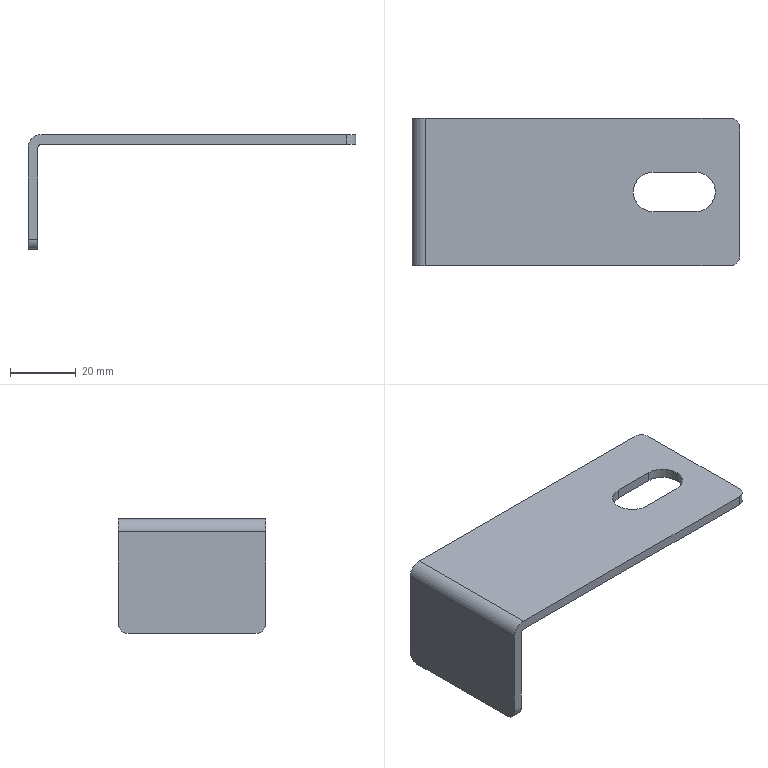Part | STEP file | 护栏FixedPlate 2-2 | 1 solid | 19 faces | box 100 x 45 x 35 mm | volume 16845 mm3 | plane 10 | cylinder 9 | commonest cylinder face diameters 6 x4 12 x3 2 x1 8 x1
STEP:
#1=CARTESIAN_POINT('',(0.,0.,0.));
#2=DIRECTION('',(0.,0.,1.));
#3=DIRECTION('',(1.,0.,0.));
#4=AXIS2_PLACEMENT_3D('',#1,#2,#3);
#5=CARTESIAN_POINT('',(73.5,6.,0.));
#6=VERTEX_POINT('',#5);
#7=CARTESIAN_POINT('',(73.5,6.,-3.));
#8=VERTEX_POINT('',#7);
#9=CARTESIAN_POINT('',(73.5,6.,-3.));
#10=DIRECTION('',(0.,0.,-1.));
#11=VECTOR('',#10,1.);
#12=LINE('',#9,#11);
#13=CARTESIAN_POINT('',(73.5,0.,-3.));
#14=DIRECTION('',(0.,0.,-1.));
#15=DIRECTION('',(-1.,0.,0.));
#16=AXIS2_PLACEMENT_3D('',#13,#14,#15);
#17=CYLINDRICAL_SURFACE('',#16,6.);
#18=CARTESIAN_POINT('',(1.571,0.));
#19=DIRECTION('',(0.,1.));
#20=VECTOR('',#19,1.);
#21=LINE('',#18,#20);
#22=(GEOMETRIC_REPRESENTATION_CONTEXT(2)PARAMETRIC_REPRESENTATION_CONTEXT()REPRESENTATION_CONTEXT('',''));
#23=DEFINITIONAL_REPRESENTATION('',(#21),#22);
#24=PCURVE('',#17,#23);
#25=CARTESIAN_POINT('',(73.5,6.,-3.));
#26=DIRECTION('',(0.,1.,0.));
#27=DIRECTION('',(-1.,0.,0.));
#28=AXIS2_PLACEMENT_3D('',#25,#26,#27);
#29=PLANE('',#28);
#30=CARTESIAN_POINT('',(0.,0.));
#31=DIRECTION('',(0.,-1.));
#32=VECTOR('',#31,1.);
#33=LINE('',#30,#32);
#34=(GEOMETRIC_REPRESENTATION_CONTEXT(2)PARAMETRIC_REPRESENTATION_CONTEXT()REPRESENTATION_CONTEXT('',''));
#35=DEFINITIONAL_REPRESENTATION('',(#33),#34);
#36=PCURVE('',#29,#35);
#37=SURFACE_CURVE('',#12,(#24,#36),.PCURVE_S1.);
#38=EDGE_CURVE('',#6,#8,#37,.T.);
#39=ORIENTED_EDGE('',*,*,#38,.T.);
#40=CARTESIAN_POINT('',(67.5,0.,-3.));
#41=VERTEX_POINT('',#40);
#42=CARTESIAN_POINT('',(73.5,0.,-3.));
#43=DIRECTION('',(0.,0.,-1.));
#44=DIRECTION('',(-1.,0.,0.));
#45=AXIS2_PLACEMENT_3D('',#42,#43,#44);
#46=CIRCLE('',#45,6.);
#47=CARTESIAN_POINT('',(0.,0.));
#48=DIRECTION('',(1.,0.));
#49=VECTOR('',#48,1.);
#50=LINE('',#47,#49);
#51=(GEOMETRIC_REPRESENTATION_CONTEXT(2)PARAMETRIC_REPRESENTATION_CONTEXT()REPRESENTATION_CONTEXT('',''));
#52=DEFINITIONAL_REPRESENTATION('',(#50),#51);
#53=PCURVE('',#17,#52);
#54=CARTESIAN_POINT('',(4.,22.5,-3.));
#55=DIRECTION('',(0.,0.,1.));
#56=DIRECTION('',(1.,0.,0.));
#57=AXIS2_PLACEMENT_3D('',#54,#55,#56);
#58=PLANE('',#57);
#59=CARTESIAN_POINT('',(63.5,-22.5));
#60=CARTESIAN_POINT('',(63.5,-12.108));
#61=CARTESIAN_POINT('',(72.5,-17.304));
#62=CARTESIAN_POINT('',(81.5,-22.5));
#63=CARTESIAN_POINT('',(72.5,-27.696));
#64=CARTESIAN_POINT('',(63.5,-32.892));
#65=CARTESIAN_POINT('',(63.5,-22.5));
#66=(BOUNDED_CURVE()B_SPLINE_CURVE(2,(#59,#60,#61,#62,#63,#64,#65),.UNSPECIFIED.,.T.,.F.)B_SPLINE_CURVE_WITH_KNOTS((1,2,2,2,2,1),(-2.094,0.,2.094,4.189,6.283,8.378),.UNSPECIFIED.)CURVE()GEOMETRIC_REPRESENTATION_ITEM()RATIONAL_B_SPLINE_CURVE((1.,0.5,1.,0.5,1.,0.5,1.))REPRESENTATION_ITEM(''));
#67=(GEOMETRIC_REPRESENTATION_CONTEXT(2)PARAMETRIC_REPRESENTATION_CONTEXT()REPRESENTATION_CONTEXT('',''));
#68=DEFINITIONAL_REPRESENTATION('',(#66),#67);
#69=PCURVE('',#58,#68);
#70=SURFACE_CURVE('',#46,(#53,#69),.PCURVE_S1.);
#71=EDGE_CURVE('',#41,#8,#70,.T.);
#72=ORIENTED_EDGE('',*,*,#71,.F.);
#73=CARTESIAN_POINT('',(67.5,0.,0.));
#74=VERTEX_POINT('',#73);
#75=CARTESIAN_POINT('',(67.5,0.,-3.));
#76=DIRECTION('',(0.,0.,-1.));
#77=VECTOR('',#76,1.);
#78=LINE('',#75,#77);
#79=CARTESIAN_POINT('',(0.,0.));
#80=DIRECTION('',(0.,1.));
#81=VECTOR('',#80,1.);
#82=LINE('',#79,#81);
#83=(GEOMETRIC_REPRESENTATION_CONTEXT(2)PARAMETRIC_REPRESENTATION_CONTEXT()REPRESENTATION_CONTEXT('',''));
#84=DEFINITIONAL_REPRESENTATION('',(#82),#83);
#85=PCURVE('',#17,#84);
#86=CARTESIAN_POINT('',(73.5,0.,-3.));
#87=DIRECTION('',(0.,0.,-1.));
#88=DIRECTION('',(-1.,0.,0.));
#89=AXIS2_PLACEMENT_3D('',#86,#87,#88);
#90=CYLINDRICAL_SURFACE('',#89,6.);
#91=CARTESIAN_POINT('',(6.283,0.));
#92=DIRECTION('',(0.,1.));
#93=VECTOR('',#92,1.);
#94=LINE('',#91,#93);
#95=(GEOMETRIC_REPRESENTATION_CONTEXT(2)PARAMETRIC_REPRESENTATION_CONTEXT()REPRESENTATION_CONTEXT('',''));
#96=DEFINITIONAL_REPRESENTATION('',(#94),#95);
#97=PCURVE('',#90,#96);
#98=SURFACE_CURVE('',#78,(#85,#97),.PCURVE_S1.);
#99=EDGE_CURVE('',#74,#41,#98,.T.);
#100=ORIENTED_EDGE('',*,*,#99,.F.);
#101=CARTESIAN_POINT('',(73.5,0.,0.));
#102=DIRECTION('',(0.,0.,1.));
#103=DIRECTION('',(1.,0.,0.));
#104=AXIS2_PLACEMENT_3D('',#101,#102,#103);
#105=CIRCLE('',#104,6.);
#106=CARTESIAN_POINT('',(3.142,-3.));
#107=DIRECTION('',(-1.,0.));
#108=VECTOR('',#107,1.);
#109=LINE('',#106,#108);
#110=(GEOMETRIC_REPRESENTATION_CONTEXT(2)PARAMETRIC_REPRESENTATION_CONTEXT()REPRESENTATION_CONTEXT('',''));
#111=DEFINITIONAL_REPRESENTATION('',(#109),#110);
#112=PCURVE('',#17,#111);
#113=CARTESIAN_POINT('',(4.,22.5,0.));
#114=DIRECTION('',(0.,0.,1.));
#115=DIRECTION('',(1.,0.,0.));
#116=AXIS2_PLACEMENT_3D('',#113,#114,#115);
#117=PLANE('',#116);
#118=CARTESIAN_POINT('',(69.5,-22.5));
#119=DIRECTION('',(1.,0.));
#120=AXIS2_PLACEMENT_2D('',#118,#119);
#121=CIRCLE('',#120,6.);
#122=(GEOMETRIC_REPRESENTATION_CONTEXT(2)PARAMETRIC_REPRESENTATION_CONTEXT()REPRESENTATION_CONTEXT('',''));
#123=DEFINITIONAL_REPRESENTATION('',(#121),#122);
#124=PCURVE('',#117,#123);
#125=SURFACE_CURVE('',#105,(#112,#124),.PCURVE_S1.);
#126=EDGE_CURVE('',#6,#74,#125,.T.);
#127=ORIENTED_EDGE('',*,*,#126,.F.);
#128=EDGE_LOOP('',(#39,#72,#100,#127));
#129=FACE_BOUND('',#128,.F.);
#130=ADVANCED_FACE('',(#129),#17,.F.);
#131=CARTESIAN_POINT('',(97.,22.5,-3.));
#132=VERTEX_POINT('',#131);
#133=CARTESIAN_POINT('',(4.,22.5,-3.));
#134=VERTEX_POINT('',#133);
#135=CARTESIAN_POINT('',(4.,22.5,-3.));
#136=DIRECTION('',(-1.,0.,0.));
#137=VECTOR('',#136,1.);
#138=LINE('',#135,#137);
#139=CARTESIAN_POINT('',(0.,0.));
#140=DIRECTION('',(-1.,0.));
#141=VECTOR('',#140,1.);
#142=LINE('',#139,#141);
#143=(GEOMETRIC_REPRESENTATION_CONTEXT(2)PARAMETRIC_REPRESENTATION_CONTEXT()REPRESENTATION_CONTEXT('',''));
#144=DEFINITIONAL_REPRESENTATION('',(#142),#143);
#145=PCURVE('',#58,#144);
#146=CARTESIAN_POINT('',(4.,22.5,-4.));
#147=DIRECTION('',(0.,-1.,0.));
#148=DIRECTION('',(-1.,0.,0.));
#149=AXIS2_PLACEMENT_3D('',#146,#147,#148);
#150=PLANE('',#149);
#151=CARTESIAN_POINT('',(0.,-1.));
#152=DIRECTION('',(1.,0.));
#153=VECTOR('',#152,1.);
#154=LINE('',#151,#153);
#155=(GEOMETRIC_REPRESENTATION_CONTEXT(2)PARAMETRIC_REPRESENTATION_CONTEXT()REPRESENTATION_CONTEXT('',''));
#156=DEFINITIONAL_REPRESENTATION('',(#154),#155);
#157=PCURVE('',#150,#156);
#158=SURFACE_CURVE('',#138,(#145,#157),.PCURVE_S1.);
#159=EDGE_CURVE('',#132,#134,#158,.T.);
#160=ORIENTED_EDGE('',*,*,#159,.F.);
#161=CARTESIAN_POINT('',(100.,19.5,-3.));
#162=VERTEX_POINT('',#161);
#163=CARTESIAN_POINT('',(97.,19.5,-3.));
#164=DIRECTION('',(0.,0.,-1.));
#165=DIRECTION('',(1.,0.,0.));
#166=AXIS2_PLACEMENT_3D('',#163,#164,#165);
#167=CIRCLE('',#166,3.);
#168=CARTESIAN_POINT('',(96.,-3.));
#169=CARTESIAN_POINT('',(96.,-8.196));
#170=CARTESIAN_POINT('',(91.5,-5.598));
#171=CARTESIAN_POINT('',(87.,-3.));
#172=CARTESIAN_POINT('',(91.5,-0.4019));
#173=CARTESIAN_POINT('',(96.,2.196));
#174=CARTESIAN_POINT('',(96.,-3.));
#175=(BOUNDED_CURVE()B_SPLINE_CURVE(2,(#168,#169,#170,#171,#172,#173,#174),.UNSPECIFIED.,.T.,.F.)B_SPLINE_CURVE_WITH_KNOTS((1,2,2,2,2,1),(-2.094,0.,2.094,4.189,6.283,8.378),.UNSPECIFIED.)CURVE()GEOMETRIC_REPRESENTATION_ITEM()RATIONAL_B_SPLINE_CURVE((1.,0.5,1.,0.5,1.,0.5,1.))REPRESENTATION_ITEM(''));
#176=(GEOMETRIC_REPRESENTATION_CONTEXT(2)PARAMETRIC_REPRESENTATION_CONTEXT()REPRESENTATION_CONTEXT('',''));
#177=DEFINITIONAL_REPRESENTATION('',(#175),#176);
#178=PCURVE('',#58,#177);
#179=CARTESIAN_POINT('',(97.,19.5,-3.));
#180=DIRECTION('',(0.,0.,-1.));
#181=DIRECTION('',(-1.,0.,0.));
#182=AXIS2_PLACEMENT_3D('',#179,#180,#181);
#183=CYLINDRICAL_SURFACE('',#182,3.);
#184=CARTESIAN_POINT('',(-3.142,0.));
#185=DIRECTION('',(1.,0.));
#186=VECTOR('',#185,1.);
#187=LINE('',#184,#186);
#188=(GEOMETRIC_REPRESENTATION_CONTEXT(2)PARAMETRIC_REPRESENTATION_CONTEXT()REPRESENTATION_CONTEXT('',''));
#189=DEFINITIONAL_REPRESENTATION('',(#187),#188);
#190=PCURVE('',#183,#189);
#191=SURFACE_CURVE('',#167,(#178,#190),.PCURVE_S1.);
#192=EDGE_CURVE('',#132,#162,#191,.T.);
#193=ORIENTED_EDGE('',*,*,#192,.T.);
#194=CARTESIAN_POINT('',(100.,-19.5,-3.));
#195=VERTEX_POINT('',#194);
#196=CARTESIAN_POINT('',(100.,22.5,-3.));
#197=DIRECTION('',(0.,-1.,0.));
#198=VECTOR('',#197,1.);
#199=LINE('',#196,#198);
#200=CARTESIAN_POINT('',(96.,0.));
#201=DIRECTION('',(0.,-1.));
#202=VECTOR('',#201,1.);
#203=LINE('',#200,#202);
#204=(GEOMETRIC_REPRESENTATION_CONTEXT(2)PARAMETRIC_REPRESENTATION_CONTEXT()REPRESENTATION_CONTEXT('',''));
#205=DEFINITIONAL_REPRESENTATION('',(#203),#204);
#206=PCURVE('',#58,#205);
#207=CARTESIAN_POINT('',(100.,22.5,-3.));
#208=DIRECTION('',(1.,0.,0.));
#209=DIRECTION('',(0.,0.,-1.));
#210=AXIS2_PLACEMENT_3D('',#207,#208,#209);
#211=PLANE('',#210);
#212=CARTESIAN_POINT('',(0.,0.));
#213=DIRECTION('',(0.,-1.));
#214=VECTOR('',#213,1.);
#215=LINE('',#212,#214);
#216=(GEOMETRIC_REPRESENTATION_CONTEXT(2)PARAMETRIC_REPRESENTATION_CONTEXT()REPRESENTATION_CONTEXT('',''));
#217=DEFINITIONAL_REPRESENTATION('',(#215),#216);
#218=PCURVE('',#211,#217);
#219=SURFACE_CURVE('',#199,(#206,#218),.PCURVE_S1.);
#220=EDGE_CURVE('',#162,#195,#219,.T.);
#221=ORIENTED_EDGE('',*,*,#220,.T.);
#222=CARTESIAN_POINT('',(97.,-22.5,-3.));
#223=VERTEX_POINT('',#222);
#224=CARTESIAN_POINT('',(97.,-19.5,-3.));
#225=DIRECTION('',(0.,0.,-1.));
#226=DIRECTION('',(1.,0.,0.));
#227=AXIS2_PLACEMENT_3D('',#224,#225,#226);
#228=CIRCLE('',#227,3.);
#229=CARTESIAN_POINT('',(96.,-42.));
#230=CARTESIAN_POINT('',(96.,-47.196));
#231=CARTESIAN_POINT('',(91.5,-44.598));
#232=CARTESIAN_POINT('',(87.,-42.));
#233=CARTESIAN_POINT('',(91.5,-39.402));
#234=CARTESIAN_POINT('',(96.,-36.804));
#235=CARTESIAN_POINT('',(96.,-42.));
#236=(BOUNDED_CURVE()B_SPLINE_CURVE(2,(#229,#230,#231,#232,#233,#234,#235),.UNSPECIFIED.,.T.,.F.)B_SPLINE_CURVE_WITH_KNOTS((1,2,2,2,2,1),(-2.094,0.,2.094,4.189,6.283,8.378),.UNSPECIFIED.)CURVE()GEOMETRIC_REPRESENTATION_ITEM()RATIONAL_B_SPLINE_CURVE((1.,0.5,1.,0.5,1.,0.5,1.))REPRESENTATION_ITEM(''));
#237=(GEOMETRIC_REPRESENTATION_CONTEXT(2)PARAMETRIC_REPRESENTATION_CONTEXT()REPRESENTATION_CONTEXT('',''));
#238=DEFINITIONAL_REPRESENTATION('',(#236),#237);
#239=PCURVE('',#58,#238);
#240=CARTESIAN_POINT('',(97.,-19.5,-4.));
#241=DIRECTION('',(0.,0.,1.));
#242=DIRECTION('',(1.,0.,0.));
#243=AXIS2_PLACEMENT_3D('',#240,#241,#242);
#244=CYLINDRICAL_SURFACE('',#243,3.);
#245=CARTESIAN_POINT('',(6.283,1.));
#246=DIRECTION('',(-1.,0.));
#247=VECTOR('',#246,1.);
#248=LINE('',#245,#247);
#249=(GEOMETRIC_REPRESENTATION_CONTEXT(2)PARAMETRIC_REPRESENTATION_CONTEXT()REPRESENTATION_CONTEXT('',''));
#250=DEFINITIONAL_REPRESENTATION('',(#248),#249);
#251=PCURVE('',#244,#250);
#252=SURFACE_CURVE('',#228,(#239,#251),.PCURVE_S1.);
#253=EDGE_CURVE('',#195,#223,#252,.T.);
#254=ORIENTED_EDGE('',*,*,#253,.T.);
#255=CARTESIAN_POINT('',(4.,-22.5,-3.));
#256=VERTEX_POINT('',#255);
#257=CARTESIAN_POINT('',(4.,-22.5,-3.));
#258=DIRECTION('',(-1.,0.,0.));
#259=VECTOR('',#258,1.);
#260=LINE('',#257,#259);
#261=CARTESIAN_POINT('',(0.,-45.));
#262=DIRECTION('',(-1.,0.));
#263=VECTOR('',#262,1.);
#264=LINE('',#261,#263);
#265=(GEOMETRIC_REPRESENTATION_CONTEXT(2)PARAMETRIC_REPRESENTATION_CONTEXT()REPRESENTATION_CONTEXT('',''));
#266=DEFINITIONAL_REPRESENTATION('',(#264),#265);
#267=PCURVE('',#58,#266);
#268=CARTESIAN_POINT('',(4.,-22.5,-4.));
#269=DIRECTION('',(0.,-1.,0.));
#270=DIRECTION('',(-1.,0.,0.));
#271=AXIS2_PLACEMENT_3D('',#268,#269,#270);
#272=PLANE('',#271);
#273=CARTESIAN_POINT('',(0.,-1.));
#274=DIRECTION('',(1.,0.));
#275=VECTOR('',#274,1.);
#276=LINE('',#273,#275);
#277=(GEOMETRIC_REPRESENTATION_CONTEXT(2)PARAMETRIC_REPRESENTATION_CONTEXT()REPRESENTATION_CONTEXT('',''));
#278=DEFINITIONAL_REPRESENTATION('',(#276),#277);
#279=PCURVE('',#272,#278);
#280=SURFACE_CURVE('',#260,(#267,#279),.PCURVE_S1.);
#281=EDGE_CURVE('',#223,#256,#280,.T.);
#282=ORIENTED_EDGE('',*,*,#281,.T.);
#283=CARTESIAN_POINT('',(4.,22.5,-3.));
#284=DIRECTION('',(0.,-1.,0.));
#285=VECTOR('',#284,1.);
#286=LINE('',#283,#285);
#287=CARTESIAN_POINT('',(0.,0.));
#288=DIRECTION('',(0.,-1.));
#289=VECTOR('',#288,1.);
#290=LINE('',#287,#289);
#291=(GEOMETRIC_REPRESENTATION_CONTEXT(2)PARAMETRIC_REPRESENTATION_CONTEXT()REPRESENTATION_CONTEXT('',''));
#292=DEFINITIONAL_REPRESENTATION('',(#290),#291);
#293=PCURVE('',#58,#292);
#294=CARTESIAN_POINT('',(4.,22.5,-4.));
#295=DIRECTION('',(0.,-1.,0.));
#296=DIRECTION('',(0.,0.,-1.));
#297=AXIS2_PLACEMENT_3D('',#294,#295,#296);
#298=CYLINDRICAL_SURFACE('',#297,1.);
#299=CARTESIAN_POINT('',(3.142,0.));
#300=DIRECTION('',(0.,1.));
#301=VECTOR('',#300,1.);
#302=LINE('',#299,#301);
#303=(GEOMETRIC_REPRESENTATION_CONTEXT(2)PARAMETRIC_REPRESENTATION_CONTEXT()REPRESENTATION_CONTEXT('',''));
#304=DEFINITIONAL_REPRESENTATION('',(#302),#303);
#305=PCURVE('',#298,#304);
#306=SURFACE_CURVE('',#286,(#293,#305),.PCURVE_S1.);
#307=EDGE_CURVE('',#134,#256,#306,.T.);
#308=ORIENTED_EDGE('',*,*,#307,.F.);
#309=EDGE_LOOP('',(#160,#193,#221,#254,#282,#308));
#310=FACE_BOUND('',#309,.T.);
#311=CARTESIAN_POINT('',(86.5,6.,-3.));
#312=VERTEX_POINT('',#311);
#313=CARTESIAN_POINT('',(73.5,6.,-3.));
#314=DIRECTION('',(1.,0.,0.));
#315=VECTOR('',#314,1.);
#316=LINE('',#313,#315);
#317=CARTESIAN_POINT('',(69.5,-16.5));
#318=DIRECTION('',(1.,0.));
#319=VECTOR('',#318,1.);
#320=LINE('',#317,#319);
#321=(GEOMETRIC_REPRESENTATION_CONTEXT(2)PARAMETRIC_REPRESENTATION_CONTEXT()REPRESENTATION_CONTEXT('',''));
#322=DEFINITIONAL_REPRESENTATION('',(#320),#321);
#323=PCURVE('',#58,#322);
#324=CARTESIAN_POINT('',(0.,0.));
#325=DIRECTION('',(-1.,0.));
#326=VECTOR('',#325,1.);
#327=LINE('',#324,#326);
#328=(GEOMETRIC_REPRESENTATION_CONTEXT(2)PARAMETRIC_REPRESENTATION_CONTEXT()REPRESENTATION_CONTEXT('',''));
#329=DEFINITIONAL_REPRESENTATION('',(#327),#328);
#330=PCURVE('',#29,#329);
#331=SURFACE_CURVE('',#316,(#323,#330),.PCURVE_S1.);
#332=EDGE_CURVE('',#8,#312,#331,.T.);
#333=ORIENTED_EDGE('',*,*,#332,.F.);
#334=ORIENTED_EDGE('',*,*,#71,.F.);
#335=CARTESIAN_POINT('',(73.5,-6.,-3.));
#336=VERTEX_POINT('',#335);
#337=CARTESIAN_POINT('',(73.5,0.,-3.));
#338=DIRECTION('',(0.,0.,-1.));
#339=DIRECTION('',(-1.,0.,0.));
#340=AXIS2_PLACEMENT_3D('',#337,#338,#339);
#341=CIRCLE('',#340,6.);
#342=CARTESIAN_POINT('',(63.5,-22.5));
#343=CARTESIAN_POINT('',(63.5,-12.108));
#344=CARTESIAN_POINT('',(72.5,-17.304));
#345=CARTESIAN_POINT('',(81.5,-22.5));
#346=CARTESIAN_POINT('',(72.5,-27.696));
#347=CARTESIAN_POINT('',(63.5,-32.892));
#348=CARTESIAN_POINT('',(63.5,-22.5));
#349=(BOUNDED_CURVE()B_SPLINE_CURVE(2,(#342,#343,#344,#345,#346,#347,#348),.UNSPECIFIED.,.T.,.F.)B_SPLINE_CURVE_WITH_KNOTS((1,2,2,2,2,1),(-2.094,0.,2.094,4.189,6.283,8.378),.UNSPECIFIED.)CURVE()GEOMETRIC_REPRESENTATION_ITEM()RATIONAL_B_SPLINE_CURVE((1.,0.5,1.,0.5,1.,0.5,1.))REPRESENTATION_ITEM(''));
#350=(GEOMETRIC_REPRESENTATION_CONTEXT(2)PARAMETRIC_REPRESENTATION_CONTEXT()REPRESENTATION_CONTEXT('',''));
#351=DEFINITIONAL_REPRESENTATION('',(#349),#350);
#352=PCURVE('',#58,#351);
#353=CARTESIAN_POINT('',(0.,0.));
#354=DIRECTION('',(1.,0.));
#355=VECTOR('',#354,1.);
#356=LINE('',#353,#355);
#357=(GEOMETRIC_REPRESENTATION_CONTEXT(2)PARAMETRIC_REPRESENTATION_CONTEXT()REPRESENTATION_CONTEXT('',''));
#358=DEFINITIONAL_REPRESENTATION('',(#356),#357);
#359=PCURVE('',#90,#358);
#360=SURFACE_CURVE('',#341,(#352,#359),.PCURVE_S1.);
#361=EDGE_CURVE('',#336,#41,#360,.T.);
#362=ORIENTED_EDGE('',*,*,#361,.F.);
#363=CARTESIAN_POINT('',(86.5,-6.,-3.));
#364=VERTEX_POINT('',#363);
#365=CARTESIAN_POINT('',(73.5,-6.,-3.));
#366=DIRECTION('',(1.,0.,0.));
#367=VECTOR('',#366,1.);
#368=LINE('',#365,#367);
#369=CARTESIAN_POINT('',(69.5,-28.5));
#370=DIRECTION('',(1.,0.));
#371=VECTOR('',#370,1.);
#372=LINE('',#369,#371);
#373=(GEOMETRIC_REPRESENTATION_CONTEXT(2)PARAMETRIC_REPRESENTATION_CONTEXT()REPRESENTATION_CONTEXT('',''));
#374=DEFINITIONAL_REPRESENTATION('',(#372),#373);
#375=PCURVE('',#58,#374);
#376=CARTESIAN_POINT('',(73.5,-6.,-3.));
#377=DIRECTION('',(0.,-1.,0.));
#378=DIRECTION('',(1.,0.,0.));
#379=AXIS2_PLACEMENT_3D('',#376,#377,#378);
#380=PLANE('',#379);
#381=CARTESIAN_POINT('',(0.,0.));
#382=DIRECTION('',(1.,0.));
#383=VECTOR('',#382,1.);
#384=LINE('',#381,#383);
#385=(GEOMETRIC_REPRESENTATION_CONTEXT(2)PARAMETRIC_REPRESENTATION_CONTEXT()REPRESENTATION_CONTEXT('',''));
#386=DEFINITIONAL_REPRESENTATION('',(#384),#385);
#387=PCURVE('',#380,#386);
#388=SURFACE_CURVE('',#368,(#375,#387),.PCURVE_S1.);
#389=EDGE_CURVE('',#336,#364,#388,.T.);
#390=ORIENTED_EDGE('',*,*,#389,.T.);
#391=CARTESIAN_POINT('',(86.5,0.,-3.));
#392=DIRECTION('',(0.,0.,-1.));
#393=DIRECTION('',(-1.,0.,0.));
#394=AXIS2_PLACEMENT_3D('',#391,#392,#393);
#395=CIRCLE('',#394,6.);
#396=CARTESIAN_POINT('',(76.5,-22.5));
#397=CARTESIAN_POINT('',(76.5,-12.108));
#398=CARTESIAN_POINT('',(85.5,-17.304));
#399=CARTESIAN_POINT('',(94.5,-22.5));
#400=CARTESIAN_POINT('',(85.5,-27.696));
#401=CARTESIAN_POINT('',(76.5,-32.892));
#402=CARTESIAN_POINT('',(76.5,-22.5));
#403=(BOUNDED_CURVE()B_SPLINE_CURVE(2,(#396,#397,#398,#399,#400,#401,#402),.UNSPECIFIED.,.T.,.F.)B_SPLINE_CURVE_WITH_KNOTS((1,2,2,2,2,1),(-2.094,0.,2.094,4.189,6.283,8.378),.UNSPECIFIED.)CURVE()GEOMETRIC_REPRESENTATION_ITEM()RATIONAL_B_SPLINE_CURVE((1.,0.5,1.,0.5,1.,0.5,1.))REPRESENTATION_ITEM(''));
#404=(GEOMETRIC_REPRESENTATION_CONTEXT(2)PARAMETRIC_REPRESENTATION_CONTEXT()REPRESENTATION_CONTEXT('',''));
#405=DEFINITIONAL_REPRESENTATION('',(#403),#404);
#406=PCURVE('',#58,#405);
#407=CARTESIAN_POINT('',(86.5,0.,-3.));
#408=DIRECTION('',(0.,0.,-1.));
#409=DIRECTION('',(-1.,0.,0.));
#410=AXIS2_PLACEMENT_3D('',#407,#408,#409);
#411=CYLINDRICAL_SURFACE('',#410,6.);
#412=CARTESIAN_POINT('',(0.,0.));
#413=DIRECTION('',(1.,0.));
#414=VECTOR('',#413,1.);
#415=LINE('',#412,#414);
#416=(GEOMETRIC_REPRESENTATION_CONTEXT(2)PARAMETRIC_REPRESENTATION_CONTEXT()REPRESENTATION_CONTEXT('',''));
#417=DEFINITIONAL_REPRESENTATION('',(#415),#416);
#418=PCURVE('',#411,#417);
#419=SURFACE_CURVE('',#395,(#406,#418),.PCURVE_S1.);
#420=EDGE_CURVE('',#312,#364,#419,.T.);
#421=ORIENTED_EDGE('',*,*,#420,.F.);
#422=EDGE_LOOP('',(#333,#334,#362,#390,#421));
#423=FACE_BOUND('',#422,.T.);
#424=ADVANCED_FACE('',(#310,#423),#58,.F.);
#425=CARTESIAN_POINT('',(3.,-22.5,-4.));
#426=VERTEX_POINT('',#425);
#427=CARTESIAN_POINT('',(3.,-22.5,-32.));
#428=VERTEX_POINT('',#427);
#429=CARTESIAN_POINT('',(3.,-22.5,-4.));
#430=DIRECTION('',(0.,0.,-1.));
#431=VECTOR('',#430,1.);
#432=LINE('',#429,#431);
#433=CARTESIAN_POINT('',(3.,22.5,-4.));
#434=DIRECTION('',(-1.,0.,0.));
#435=DIRECTION('',(0.,0.,1.));
#436=AXIS2_PLACEMENT_3D('',#433,#434,#435);
#437=PLANE('',#436);
#438=CARTESIAN_POINT('',(0.,-45.));
#439=DIRECTION('',(-1.,0.));
#440=VECTOR('',#439,1.);
#441=LINE('',#438,#440);
#442=(GEOMETRIC_REPRESENTATION_CONTEXT(2)PARAMETRIC_REPRESENTATION_CONTEXT()REPRESENTATION_CONTEXT('',''));
#443=DEFINITIONAL_REPRESENTATION('',(#441),#442);
#444=PCURVE('',#437,#443);
#445=CARTESIAN_POINT('',(1.,0.));
#446=DIRECTION('',(0.,1.));
#447=VECTOR('',#446,1.);
#448=LINE('',#445,#447);
#449=(GEOMETRIC_REPRESENTATION_CONTEXT(2)PARAMETRIC_REPRESENTATION_CONTEXT()REPRESENTATION_CONTEXT('',''));
#450=DEFINITIONAL_REPRESENTATION('',(#448),#449);
#451=PCURVE('',#272,#450);
#452=SURFACE_CURVE('',#432,(#444,#451),.PCURVE_S1.);
#453=EDGE_CURVE('',#426,#428,#452,.T.);
#454=ORIENTED_EDGE('',*,*,#453,.T.);
#455=CARTESIAN_POINT('',(3.,-19.5,-35.));
#456=VERTEX_POINT('',#455);
#457=CARTESIAN_POINT('',(3.,-19.5,-32.));
#458=DIRECTION('',(1.,0.,0.));
#459=DIRECTION('',(0.,0.,1.));
#460=AXIS2_PLACEMENT_3D('',#457,#458,#459);
#461=CIRCLE('',#460,3.);
#462=CARTESIAN_POINT('',(-25.,-42.));
#463=CARTESIAN_POINT('',(-25.,-47.196));
#464=CARTESIAN_POINT('',(-29.5,-44.598));
#465=CARTESIAN_POINT('',(-34.,-42.));
#466=CARTESIAN_POINT('',(-29.5,-39.402));
#467=CARTESIAN_POINT('',(-25.,-36.804));
#468=CARTESIAN_POINT('',(-25.,-42.));
#469=(BOUNDED_CURVE()B_SPLINE_CURVE(2,(#462,#463,#464,#465,#466,#467,#468),.UNSPECIFIED.,.T.,.F.)B_SPLINE_CURVE_WITH_KNOTS((1,2,2,2,2,1),(-2.094,0.,2.094,4.189,6.283,8.378),.UNSPECIFIED.)CURVE()GEOMETRIC_REPRESENTATION_ITEM()RATIONAL_B_SPLINE_CURVE((1.,0.5,1.,0.5,1.,0.5,1.))REPRESENTATION_ITEM(''));
#470=(GEOMETRIC_REPRESENTATION_CONTEXT(2)PARAMETRIC_REPRESENTATION_CONTEXT()REPRESENTATION_CONTEXT('',''));
#471=DEFINITIONAL_REPRESENTATION('',(#469),#470);
#472=PCURVE('',#437,#471);
#473=CARTESIAN_POINT('',(4.,-19.5,-32.));
#474=DIRECTION('',(1.,0.,0.));
#475=DIRECTION('',(0.,0.,-1.));
#476=AXIS2_PLACEMENT_3D('',#473,#474,#475);
#477=CYLINDRICAL_SURFACE('',#476,3.);
#478=CARTESIAN_POINT('',(3.142,-1.));
#479=DIRECTION('',(1.,0.));
#480=VECTOR('',#479,1.);
#481=LINE('',#478,#480);
#482=(GEOMETRIC_REPRESENTATION_CONTEXT(2)PARAMETRIC_REPRESENTATION_CONTEXT()REPRESENTATION_CONTEXT('',''));
#483=DEFINITIONAL_REPRESENTATION('',(#481),#482);
#484=PCURVE('',#477,#483);
#485=SURFACE_CURVE('',#461,(#472,#484),.PCURVE_S1.);
#486=EDGE_CURVE('',#428,#456,#485,.T.);
#487=ORIENTED_EDGE('',*,*,#486,.T.);
#488=CARTESIAN_POINT('',(3.,19.5,-35.));
#489=VERTEX_POINT('',#488);
#490=CARTESIAN_POINT('',(3.,22.5,-35.));
#491=DIRECTION('',(0.,-1.,0.));
#492=VECTOR('',#491,1.);
#493=LINE('',#490,#492);
#494=CARTESIAN_POINT('',(-31.,0.));
#495=DIRECTION('',(0.,-1.));
#496=VECTOR('',#495,1.);
#497=LINE('',#494,#496);
#498=(GEOMETRIC_REPRESENTATION_CONTEXT(2)PARAMETRIC_REPRESENTATION_CONTEXT()REPRESENTATION_CONTEXT('',''));
#499=DEFINITIONAL_REPRESENTATION('',(#497),#498);
#500=PCURVE('',#437,#499);
#501=CARTESIAN_POINT('',(0.,22.5,-35.));
#502=DIRECTION('',(0.,0.,-1.));
#503=DIRECTION('',(-1.,0.,0.));
#504=AXIS2_PLACEMENT_3D('',#501,#502,#503);
#505=PLANE('',#504);
#506=CARTESIAN_POINT('',(-3.,0.));
#507=DIRECTION('',(0.,-1.));
#508=VECTOR('',#507,1.);
#509=LINE('',#506,#508);
#510=(GEOMETRIC_REPRESENTATION_CONTEXT(2)PARAMETRIC_REPRESENTATION_CONTEXT()REPRESENTATION_CONTEXT('',''));
#511=DEFINITIONAL_REPRESENTATION('',(#509),#510);
#512=PCURVE('',#505,#511);
#513=SURFACE_CURVE('',#493,(#500,#512),.PCURVE_S1.);
#514=EDGE_CURVE('',#489,#456,#513,.T.);
#515=ORIENTED_EDGE('',*,*,#514,.F.);
#516=CARTESIAN_POINT('',(3.,22.5,-32.));
#517=VERTEX_POINT('',#516);
#518=CARTESIAN_POINT('',(3.,19.5,-32.));
#519=DIRECTION('',(1.,0.,0.));
#520=DIRECTION('',(0.,0.,1.));
#521=AXIS2_PLACEMENT_3D('',#518,#519,#520);
#522=CIRCLE('',#521,3.);
#523=CARTESIAN_POINT('',(-25.,-3.));
#524=CARTESIAN_POINT('',(-25.,-8.196));
#525=CARTESIAN_POINT('',(-29.5,-5.598));
#526=CARTESIAN_POINT('',(-34.,-3.));
#527=CARTESIAN_POINT('',(-29.5,-0.4019));
#528=CARTESIAN_POINT('',(-25.,2.196));
#529=CARTESIAN_POINT('',(-25.,-3.));
#530=(BOUNDED_CURVE()B_SPLINE_CURVE(2,(#523,#524,#525,#526,#527,#528,#529),.UNSPECIFIED.,.T.,.F.)B_SPLINE_CURVE_WITH_KNOTS((1,2,2,2,2,1),(-2.094,0.,2.094,4.189,6.283,8.378),.UNSPECIFIED.)CURVE()GEOMETRIC_REPRESENTATION_ITEM()RATIONAL_B_SPLINE_CURVE((1.,0.5,1.,0.5,1.,0.5,1.))REPRESENTATION_ITEM(''));
#531=(GEOMETRIC_REPRESENTATION_CONTEXT(2)PARAMETRIC_REPRESENTATION_CONTEXT()REPRESENTATION_CONTEXT('',''));
#532=DEFINITIONAL_REPRESENTATION('',(#530),#531);
#533=PCURVE('',#437,#532);
#534=CARTESIAN_POINT('',(0.,19.5,-32.));
#535=DIRECTION('',(-1.,0.,0.));
#536=DIRECTION('',(0.,0.,1.));
#537=AXIS2_PLACEMENT_3D('',#534,#535,#536);
#538=CYLINDRICAL_SURFACE('',#537,3.);
#539=CARTESIAN_POINT('',(6.283,-3.));
#540=DIRECTION('',(-1.,0.));
#541=VECTOR('',#540,1.);
#542=LINE('',#539,#541);
#543=(GEOMETRIC_REPRESENTATION_CONTEXT(2)PARAMETRIC_REPRESENTATION_CONTEXT()REPRESENTATION_CONTEXT('',''));
#544=DEFINITIONAL_REPRESENTATION('',(#542),#543);
#545=PCURVE('',#538,#544);
#546=SURFACE_CURVE('',#522,(#533,#545),.PCURVE_S1.);
#547=EDGE_CURVE('',#489,#517,#546,.T.);
#548=ORIENTED_EDGE('',*,*,#547,.T.);
#549=CARTESIAN_POINT('',(3.,22.5,-4.));
#550=VERTEX_POINT('',#549);
#551=CARTESIAN_POINT('',(3.,22.5,-4.));
#552=DIRECTION('',(0.,0.,-1.));
#553=VECTOR('',#552,1.);
#554=LINE('',#551,#553);
#555=CARTESIAN_POINT('',(0.,0.));
#556=DIRECTION('',(-1.,0.));
#557=VECTOR('',#556,1.);
#558=LINE('',#555,#557);
#559=(GEOMETRIC_REPRESENTATION_CONTEXT(2)PARAMETRIC_REPRESENTATION_CONTEXT()REPRESENTATION_CONTEXT('',''));
#560=DEFINITIONAL_REPRESENTATION('',(#558),#559);
#561=PCURVE('',#437,#560);
#562=CARTESIAN_POINT('',(1.,0.));
#563=DIRECTION('',(0.,1.));
#564=VECTOR('',#563,1.);
#565=LINE('',#562,#564);
#566=(GEOMETRIC_REPRESENTATION_CONTEXT(2)PARAMETRIC_REPRESENTATION_CONTEXT()REPRESENTATION_CONTEXT('',''));
#567=DEFINITIONAL_REPRESENTATION('',(#565),#566);
#568=PCURVE('',#150,#567);
#569=SURFACE_CURVE('',#554,(#561,#568),.PCURVE_S1.);
#570=EDGE_CURVE('',#550,#517,#569,.T.);
#571=ORIENTED_EDGE('',*,*,#570,.F.);
#572=CARTESIAN_POINT('',(3.,22.5,-4.));
#573=DIRECTION('',(0.,-1.,0.));
#574=VECTOR('',#573,1.);
#575=LINE('',#572,#574);
#576=CARTESIAN_POINT('',(0.,0.));
#577=DIRECTION('',(0.,-1.));
#578=VECTOR('',#577,1.);
#579=LINE('',#576,#578);
#580=(GEOMETRIC_REPRESENTATION_CONTEXT(2)PARAMETRIC_REPRESENTATION_CONTEXT()REPRESENTATION_CONTEXT('',''));
#581=DEFINITIONAL_REPRESENTATION('',(#579),#580);
#582=PCURVE('',#437,#581);
#583=CARTESIAN_POINT('',(4.712,0.));
#584=DIRECTION('',(0.,1.));
#585=VECTOR('',#584,1.);
#586=LINE('',#583,#585);
#587=(GEOMETRIC_REPRESENTATION_CONTEXT(2)PARAMETRIC_REPRESENTATION_CONTEXT()REPRESENTATION_CONTEXT('',''));
#588=DEFINITIONAL_REPRESENTATION('',(#586),#587);
#589=PCURVE('',#298,#588);
#590=SURFACE_CURVE('',#575,(#582,#589),.PCURVE_S1.);
#591=EDGE_CURVE('',#550,#426,#590,.T.);
#592=ORIENTED_EDGE('',*,*,#591,.T.);
#593=EDGE_LOOP('',(#454,#487,#515,#548,#571,#592));
#594=FACE_BOUND('',#593,.T.);
#595=ADVANCED_FACE('',(#594),#437,.F.);
#596=ORIENTED_EDGE('',*,*,#514,.T.);
#597=CARTESIAN_POINT('',(0.,-19.5,-35.));
#598=VERTEX_POINT('',#597);
#599=CARTESIAN_POINT('',(0.,-19.5,-35.));
#600=DIRECTION('',(-1.,0.,0.));
#601=VECTOR('',#600,1.);
#602=LINE('',#599,#601);
#603=CARTESIAN_POINT('',(0.,-42.));
#604=DIRECTION('',(1.,0.));
#605=VECTOR('',#604,1.);
#606=LINE('',#603,#605);
#607=(GEOMETRIC_REPRESENTATION_CONTEXT(2)PARAMETRIC_REPRESENTATION_CONTEXT()REPRESENTATION_CONTEXT('',''));
#608=DEFINITIONAL_REPRESENTATION('',(#606),#607);
#609=PCURVE('',#505,#608);
#610=CARTESIAN_POINT('',(6.283,-4.));
#611=DIRECTION('',(0.,-1.));
#612=VECTOR('',#611,1.);
#613=LINE('',#610,#612);
#614=(GEOMETRIC_REPRESENTATION_CONTEXT(2)PARAMETRIC_REPRESENTATION_CONTEXT()REPRESENTATION_CONTEXT('',''));
#615=DEFINITIONAL_REPRESENTATION('',(#613),#614);
#616=PCURVE('',#477,#615);
#617=SURFACE_CURVE('',#602,(#609,#616),.PCURVE_S1.);
#618=EDGE_CURVE('',#456,#598,#617,.T.);
#619=ORIENTED_EDGE('',*,*,#618,.T.);
#620=CARTESIAN_POINT('',(0.,19.5,-35.));
#621=VERTEX_POINT('',#620);
#622=CARTESIAN_POINT('',(0.,22.5,-35.));
#623=DIRECTION('',(0.,-1.,0.));
#624=VECTOR('',#623,1.);
#625=LINE('',#622,#624);
#626=CARTESIAN_POINT('',(0.,0.));
#627=DIRECTION('',(0.,-1.));
#628=VECTOR('',#627,1.);
#629=LINE('',#626,#628);
#630=(GEOMETRIC_REPRESENTATION_CONTEXT(2)PARAMETRIC_REPRESENTATION_CONTEXT()REPRESENTATION_CONTEXT('',''));
#631=DEFINITIONAL_REPRESENTATION('',(#629),#630);
#632=PCURVE('',#505,#631);
#633=CARTESIAN_POINT('',(0.,22.5,-4.));
#634=DIRECTION('',(-1.,0.,0.));
#635=DIRECTION('',(0.,0.,1.));
#636=AXIS2_PLACEMENT_3D('',#633,#634,#635);
#637=PLANE('',#636);
#638=CARTESIAN_POINT('',(-31.,0.));
#639=DIRECTION('',(0.,-1.));
#640=VECTOR('',#639,1.);
#641=LINE('',#638,#640);
#642=(GEOMETRIC_REPRESENTATION_CONTEXT(2)PARAMETRIC_REPRESENTATION_CONTEXT()REPRESENTATION_CONTEXT('',''));
#643=DEFINITIONAL_REPRESENTATION('',(#641),#642);
#644=PCURVE('',#637,#643);
#645=SURFACE_CURVE('',#625,(#632,#644),.PCURVE_S1.);
#646=EDGE_CURVE('',#621,#598,#645,.T.);
#647=ORIENTED_EDGE('',*,*,#646,.F.);
#648=CARTESIAN_POINT('',(3.,19.5,-35.));
#649=DIRECTION('',(1.,0.,0.));
#650=VECTOR('',#649,1.);
#651=LINE('',#648,#650);
#652=CARTESIAN_POINT('',(-3.,-3.));
#653=DIRECTION('',(-1.,0.));
#654=VECTOR('',#653,1.);
#655=LINE('',#652,#654);
#656=(GEOMETRIC_REPRESENTATION_CONTEXT(2)PARAMETRIC_REPRESENTATION_CONTEXT()REPRESENTATION_CONTEXT('',''));
#657=DEFINITIONAL_REPRESENTATION('',(#655),#656);
#658=PCURVE('',#505,#657);
#659=CARTESIAN_POINT('',(3.142,-3.));
#660=DIRECTION('',(0.,-1.));
#661=VECTOR('',#660,1.);
#662=LINE('',#659,#661);
#663=(GEOMETRIC_REPRESENTATION_CONTEXT(2)PARAMETRIC_REPRESENTATION_CONTEXT()REPRESENTATION_CONTEXT('',''));
#664=DEFINITIONAL_REPRESENTATION('',(#662),#663);
#665=PCURVE('',#538,#664);
#666=SURFACE_CURVE('',#651,(#658,#665),.PCURVE_S1.);
#667=EDGE_CURVE('',#621,#489,#666,.T.);
#668=ORIENTED_EDGE('',*,*,#667,.T.);
#669=EDGE_LOOP('',(#596,#619,#647,#668));
#670=FACE_BOUND('',#669,.T.);
#671=ADVANCED_FACE('',(#670),#505,.T.);
#672=ORIENTED_EDGE('',*,*,#646,.T.);
#673=CARTESIAN_POINT('',(0.,-22.5,-32.));
#674=VERTEX_POINT('',#673);
#675=CARTESIAN_POINT('',(0.,-19.5,-32.));
#676=DIRECTION('',(-1.,0.,0.));
#677=DIRECTION('',(0.,0.,1.));
#678=AXIS2_PLACEMENT_3D('',#675,#676,#677);
#679=CIRCLE('',#678,3.);
#680=CARTESIAN_POINT('',(-28.,-42.));
#681=DIRECTION('',(1.,0.));
#682=AXIS2_PLACEMENT_2D('',#680,#681);
#683=CIRCLE('',#682,3.);
#684=(GEOMETRIC_REPRESENTATION_CONTEXT(2)PARAMETRIC_REPRESENTATION_CONTEXT()REPRESENTATION_CONTEXT('',''));
#685=DEFINITIONAL_REPRESENTATION('',(#683),#684);
#686=PCURVE('',#637,#685);
#687=CARTESIAN_POINT('',(9.425,-4.));
#688=DIRECTION('',(-1.,0.));
#689=VECTOR('',#688,1.);
#690=LINE('',#687,#689);
#691=(GEOMETRIC_REPRESENTATION_CONTEXT(2)PARAMETRIC_REPRESENTATION_CONTEXT()REPRESENTATION_CONTEXT('',''));
#692=DEFINITIONAL_REPRESENTATION('',(#690),#691);
#693=PCURVE('',#477,#692);
#694=SURFACE_CURVE('',#679,(#686,#693),.PCURVE_S1.);
#695=EDGE_CURVE('',#598,#674,#694,.T.);
#696=ORIENTED_EDGE('',*,*,#695,.T.);
#697=CARTESIAN_POINT('',(0.,-22.5,-4.));
#698=VERTEX_POINT('',#697);
#699=CARTESIAN_POINT('',(0.,-22.5,-4.));
#700=DIRECTION('',(0.,0.,-1.));
#701=VECTOR('',#700,1.);
#702=LINE('',#699,#701);
#703=CARTESIAN_POINT('',(0.,-45.));
#704=DIRECTION('',(-1.,0.));
#705=VECTOR('',#704,1.);
#706=LINE('',#703,#705);
#707=(GEOMETRIC_REPRESENTATION_CONTEXT(2)PARAMETRIC_REPRESENTATION_CONTEXT()REPRESENTATION_CONTEXT('',''));
#708=DEFINITIONAL_REPRESENTATION('',(#706),#707);
#709=PCURVE('',#637,#708);
#710=CARTESIAN_POINT('',(4.,0.));
#711=DIRECTION('',(0.,1.));
#712=VECTOR('',#711,1.);
#713=LINE('',#710,#712);
#714=(GEOMETRIC_REPRESENTATION_CONTEXT(2)PARAMETRIC_REPRESENTATION_CONTEXT()REPRESENTATION_CONTEXT('',''));
#715=DEFINITIONAL_REPRESENTATION('',(#713),#714);
#716=PCURVE('',#272,#715);
#717=SURFACE_CURVE('',#702,(#709,#716),.PCURVE_S1.);
#718=EDGE_CURVE('',#698,#674,#717,.T.);
#719=ORIENTED_EDGE('',*,*,#718,.F.);
#720=CARTESIAN_POINT('',(0.,22.5,-4.));
#721=VERTEX_POINT('',#720);
#722=CARTESIAN_POINT('',(0.,22.5,-4.));
#723=DIRECTION('',(0.,-1.,0.));
#724=VECTOR('',#723,1.);
#725=LINE('',#722,#724);
#726=CARTESIAN_POINT('',(0.,0.));
#727=DIRECTION('',(0.,-1.));
#728=VECTOR('',#727,1.);
#729=LINE('',#726,#728);
#730=(GEOMETRIC_REPRESENTATION_CONTEXT(2)PARAMETRIC_REPRESENTATION_CONTEXT()REPRESENTATION_CONTEXT('',''));
#731=DEFINITIONAL_REPRESENTATION('',(#729),#730);
#732=PCURVE('',#637,#731);
#733=CARTESIAN_POINT('',(4.,22.5,-4.));
#734=DIRECTION('',(0.,-1.,0.));
#735=DIRECTION('',(0.,0.,-1.));
#736=AXIS2_PLACEMENT_3D('',#733,#734,#735);
#737=CYLINDRICAL_SURFACE('',#736,4.);
#738=CARTESIAN_POINT('',(4.712,0.));
#739=DIRECTION('',(0.,1.));
#740=VECTOR('',#739,1.);
#741=LINE('',#738,#740);
#742=(GEOMETRIC_REPRESENTATION_CONTEXT(2)PARAMETRIC_REPRESENTATION_CONTEXT()REPRESENTATION_CONTEXT('',''));
#743=DEFINITIONAL_REPRESENTATION('',(#741),#742);
#744=PCURVE('',#737,#743);
#745=SURFACE_CURVE('',#725,(#732,#744),.PCURVE_S1.);
#746=EDGE_CURVE('',#721,#698,#745,.T.);
#747=ORIENTED_EDGE('',*,*,#746,.F.);
#748=CARTESIAN_POINT('',(0.,22.5,-32.));
#749=VERTEX_POINT('',#748);
#750=CARTESIAN_POINT('',(0.,22.5,-4.));
#751=DIRECTION('',(0.,0.,-1.));
#752=VECTOR('',#751,1.);
#753=LINE('',#750,#752);
#754=CARTESIAN_POINT('',(0.,0.));
#755=DIRECTION('',(-1.,0.));
#756=VECTOR('',#755,1.);
#757=LINE('',#754,#756);
#758=(GEOMETRIC_REPRESENTATION_CONTEXT(2)PARAMETRIC_REPRESENTATION_CONTEXT()REPRESENTATION_CONTEXT('',''));
#759=DEFINITIONAL_REPRESENTATION('',(#757),#758);
#760=PCURVE('',#637,#759);
#761=CARTESIAN_POINT('',(4.,0.));
#762=DIRECTION('',(0.,1.));
#763=VECTOR('',#762,1.);
#764=LINE('',#761,#763);
#765=(GEOMETRIC_REPRESENTATION_CONTEXT(2)PARAMETRIC_REPRESENTATION_CONTEXT()REPRESENTATION_CONTEXT('',''));
#766=DEFINITIONAL_REPRESENTATION('',(#764),#765);
#767=PCURVE('',#150,#766);
#768=SURFACE_CURVE('',#753,(#760,#767),.PCURVE_S1.);
#769=EDGE_CURVE('',#721,#749,#768,.T.);
#770=ORIENTED_EDGE('',*,*,#769,.T.);
#771=CARTESIAN_POINT('',(0.,19.5,-32.));
#772=DIRECTION('',(-1.,0.,0.));
#773=DIRECTION('',(0.,0.,1.));
#774=AXIS2_PLACEMENT_3D('',#771,#772,#773);
#775=CIRCLE('',#774,3.);
#776=CARTESIAN_POINT('',(-28.,-3.));
#777=DIRECTION('',(1.,0.));
#778=AXIS2_PLACEMENT_2D('',#776,#777);
#779=CIRCLE('',#778,3.);
#780=(GEOMETRIC_REPRESENTATION_CONTEXT(2)PARAMETRIC_REPRESENTATION_CONTEXT()REPRESENTATION_CONTEXT('',''));
#781=DEFINITIONAL_REPRESENTATION('',(#779),#780);
#782=PCURVE('',#637,#781);
#783=CARTESIAN_POINT('',(0.,0.));
#784=DIRECTION('',(1.,0.));
#785=VECTOR('',#784,1.);
#786=LINE('',#783,#785);
#787=(GEOMETRIC_REPRESENTATION_CONTEXT(2)PARAMETRIC_REPRESENTATION_CONTEXT()REPRESENTATION_CONTEXT('',''));
#788=DEFINITIONAL_REPRESENTATION('',(#786),#787);
#789=PCURVE('',#538,#788);
#790=SURFACE_CURVE('',#775,(#782,#789),.PCURVE_S1.);
#791=EDGE_CURVE('',#749,#621,#790,.T.);
#792=ORIENTED_EDGE('',*,*,#791,.T.);
#793=EDGE_LOOP('',(#672,#696,#719,#747,#770,#792));
#794=FACE_BOUND('',#793,.T.);
#795=ADVANCED_FACE('',(#794),#637,.T.);
#796=CARTESIAN_POINT('',(4.,-22.5,0.));
#797=VERTEX_POINT('',#796);
#798=CARTESIAN_POINT('',(4.,-22.5,-4.));
#799=DIRECTION('',(0.,-1.,0.));
#800=DIRECTION('',(0.,0.,-1.));
#801=AXIS2_PLACEMENT_3D('',#798,#799,#800);
#802=CIRCLE('',#801,4.);
#803=CARTESIAN_POINT('',(0.,45.));
#804=DIRECTION('',(1.,0.));
#805=VECTOR('',#804,1.);
#806=LINE('',#803,#805);
#807=(GEOMETRIC_REPRESENTATION_CONTEXT(2)PARAMETRIC_REPRESENTATION_CONTEXT()REPRESENTATION_CONTEXT('',''));
#808=DEFINITIONAL_REPRESENTATION('',(#806),#807);
#809=PCURVE('',#737,#808);
#810=CARTESIAN_POINT('',(0.,0.));
#811=DIRECTION('',(0.,1.));
#812=AXIS2_PLACEMENT_2D('',#810,#811);
#813=CIRCLE('',#812,4.);
#814=(GEOMETRIC_REPRESENTATION_CONTEXT(2)PARAMETRIC_REPRESENTATION_CONTEXT()REPRESENTATION_CONTEXT('',''));
#815=DEFINITIONAL_REPRESENTATION('',(#813),#814);
#816=PCURVE('',#272,#815);
#817=SURFACE_CURVE('',#802,(#809,#816),.PCURVE_S1.);
#818=EDGE_CURVE('',#797,#698,#817,.T.);
#819=ORIENTED_EDGE('',*,*,#818,.F.);
#820=CARTESIAN_POINT('',(4.,22.5,0.));
#821=VERTEX_POINT('',#820);
#822=CARTESIAN_POINT('',(4.,22.5,0.));
#823=DIRECTION('',(0.,-1.,0.));
#824=VECTOR('',#823,1.);
#825=LINE('',#822,#824);
#826=CARTESIAN_POINT('',(3.142,0.));
#827=DIRECTION('',(0.,1.));
#828=VECTOR('',#827,1.);
#829=LINE('',#826,#828);
#830=(GEOMETRIC_REPRESENTATION_CONTEXT(2)PARAMETRIC_REPRESENTATION_CONTEXT()REPRESENTATION_CONTEXT('',''));
#831=DEFINITIONAL_REPRESENTATION('',(#829),#830);
#832=PCURVE('',#737,#831);
#833=CARTESIAN_POINT('',(0.,0.));
#834=DIRECTION('',(0.,-1.));
#835=VECTOR('',#834,1.);
#836=LINE('',#833,#835);
#837=(GEOMETRIC_REPRESENTATION_CONTEXT(2)PARAMETRIC_REPRESENTATION_CONTEXT()REPRESENTATION_CONTEXT('',''));
#838=DEFINITIONAL_REPRESENTATION('',(#836),#837);
#839=PCURVE('',#117,#838);
#840=SURFACE_CURVE('',#825,(#832,#839),.PCURVE_S1.);
#841=EDGE_CURVE('',#821,#797,#840,.T.);
#842=ORIENTED_EDGE('',*,*,#841,.F.);
#843=CARTESIAN_POINT('',(4.,22.5,-4.));
#844=DIRECTION('',(0.,-1.,0.));
#845=DIRECTION('',(0.,0.,-1.));
#846=AXIS2_PLACEMENT_3D('',#843,#844,#845);
#847=CIRCLE('',#846,4.);
#848=CARTESIAN_POINT('',(0.,0.));
#849=DIRECTION('',(1.,0.));
#850=VECTOR('',#849,1.);
#851=LINE('',#848,#850);
#852=(GEOMETRIC_REPRESENTATION_CONTEXT(2)PARAMETRIC_REPRESENTATION_CONTEXT()REPRESENTATION_CONTEXT('',''));
#853=DEFINITIONAL_REPRESENTATION('',(#851),#852);
#854=PCURVE('',#737,#853);
#855=CARTESIAN_POINT('',(0.,0.));
#856=DIRECTION('',(0.,1.));
#857=AXIS2_PLACEMENT_2D('',#855,#856);
#858=CIRCLE('',#857,4.);
#859=(GEOMETRIC_REPRESENTATION_CONTEXT(2)PARAMETRIC_REPRESENTATION_CONTEXT()REPRESENTATION_CONTEXT('',''));
#860=DEFINITIONAL_REPRESENTATION('',(#858),#859);
#861=PCURVE('',#150,#860);
#862=SURFACE_CURVE('',#847,(#854,#861),.PCURVE_S1.);
#863=EDGE_CURVE('',#821,#721,#862,.T.);
#864=ORIENTED_EDGE('',*,*,#863,.T.);
#865=ORIENTED_EDGE('',*,*,#746,.T.);
#866=EDGE_LOOP('',(#819,#842,#864,#865));
#867=FACE_BOUND('',#866,.T.);
#868=ADVANCED_FACE('',(#867),#737,.T.);
#869=ORIENTED_EDGE('',*,*,#126,.F.);
#870=CARTESIAN_POINT('',(86.5,6.,0.));
#871=VERTEX_POINT('',#870);
#872=CARTESIAN_POINT('',(4.,6.,0.));
#873=DIRECTION('',(-1.,0.,0.));
#874=VECTOR('',#873,1.);
#875=LINE('',#872,#874);
#876=CARTESIAN_POINT('',(0.,-16.5));
#877=DIRECTION('',(-1.,0.));
#878=VECTOR('',#877,1.);
#879=LINE('',#876,#878);
#880=(GEOMETRIC_REPRESENTATION_CONTEXT(2)PARAMETRIC_REPRESENTATION_CONTEXT()REPRESENTATION_CONTEXT('',''));
#881=DEFINITIONAL_REPRESENTATION('',(#879),#880);
#882=PCURVE('',#117,#881);
#883=CARTESIAN_POINT('',(69.5,3.));
#884=DIRECTION('',(1.,0.));
#885=VECTOR('',#884,1.);
#886=LINE('',#883,#885);
#887=(GEOMETRIC_REPRESENTATION_CONTEXT(2)PARAMETRIC_REPRESENTATION_CONTEXT()REPRESENTATION_CONTEXT('',''));
#888=DEFINITIONAL_REPRESENTATION('',(#886),#887);
#889=PCURVE('',#29,#888);
#890=SURFACE_CURVE('',#875,(#882,#889),.PCURVE_S1.);
#891=EDGE_CURVE('',#871,#6,#890,.T.);
#892=ORIENTED_EDGE('',*,*,#891,.F.);
#893=CARTESIAN_POINT('',(86.5,-6.,0.));
#894=VERTEX_POINT('',#893);
#895=CARTESIAN_POINT('',(86.5,0.,0.));
#896=DIRECTION('',(0.,0.,1.));
#897=DIRECTION('',(1.,0.,0.));
#898=AXIS2_PLACEMENT_3D('',#895,#896,#897);
#899=CIRCLE('',#898,6.);
#900=CARTESIAN_POINT('',(82.5,-22.5));
#901=DIRECTION('',(1.,0.));
#902=AXIS2_PLACEMENT_2D('',#900,#901);
#903=CIRCLE('',#902,6.);
#904=(GEOMETRIC_REPRESENTATION_CONTEXT(2)PARAMETRIC_REPRESENTATION_CONTEXT()REPRESENTATION_CONTEXT('',''));
#905=DEFINITIONAL_REPRESENTATION('',(#903),#904);
#906=PCURVE('',#117,#905);
#907=CARTESIAN_POINT('',(9.425,-3.));
#908=DIRECTION('',(-1.,0.));
#909=VECTOR('',#908,1.);
#910=LINE('',#907,#909);
#911=(GEOMETRIC_REPRESENTATION_CONTEXT(2)PARAMETRIC_REPRESENTATION_CONTEXT()REPRESENTATION_CONTEXT('',''));
#912=DEFINITIONAL_REPRESENTATION('',(#910),#911);
#913=PCURVE('',#411,#912);
#914=SURFACE_CURVE('',#899,(#906,#913),.PCURVE_S1.);
#915=EDGE_CURVE('',#894,#871,#914,.T.);
#916=ORIENTED_EDGE('',*,*,#915,.F.);
#917=CARTESIAN_POINT('',(73.5,-6.,0.));
#918=VERTEX_POINT('',#917);
#919=CARTESIAN_POINT('',(4.,-6.,0.));
#920=DIRECTION('',(1.,0.,0.));
#921=VECTOR('',#920,1.);
#922=LINE('',#919,#921);
#923=CARTESIAN_POINT('',(0.,-28.5));
#924=DIRECTION('',(1.,0.));
#925=VECTOR('',#924,1.);
#926=LINE('',#923,#925);
#927=(GEOMETRIC_REPRESENTATION_CONTEXT(2)PARAMETRIC_REPRESENTATION_CONTEXT()REPRESENTATION_CONTEXT('',''));
#928=DEFINITIONAL_REPRESENTATION('',(#926),#927);
#929=PCURVE('',#117,#928);
#930=CARTESIAN_POINT('',(-69.5,3.));
#931=DIRECTION('',(1.,0.));
#932=VECTOR('',#931,1.);
#933=LINE('',#930,#932);
#934=(GEOMETRIC_REPRESENTATION_CONTEXT(2)PARAMETRIC_REPRESENTATION_CONTEXT()REPRESENTATION_CONTEXT('',''));
#935=DEFINITIONAL_REPRESENTATION('',(#933),#934);
#936=PCURVE('',#380,#935);
#937=SURFACE_CURVE('',#922,(#929,#936),.PCURVE_S1.);
#938=EDGE_CURVE('',#918,#894,#937,.T.);
#939=ORIENTED_EDGE('',*,*,#938,.F.);
#940=CARTESIAN_POINT('',(73.5,0.,0.));
#941=DIRECTION('',(0.,0.,1.));
#942=DIRECTION('',(1.,0.,0.));
#943=AXIS2_PLACEMENT_3D('',#940,#941,#942);
#944=CIRCLE('',#943,6.);
#945=CARTESIAN_POINT('',(69.5,-22.5));
#946=DIRECTION('',(1.,0.));
#947=AXIS2_PLACEMENT_2D('',#945,#946);
#948=CIRCLE('',#947,6.);
#949=(GEOMETRIC_REPRESENTATION_CONTEXT(2)PARAMETRIC_REPRESENTATION_CONTEXT()REPRESENTATION_CONTEXT('',''));
#950=DEFINITIONAL_REPRESENTATION('',(#948),#949);
#951=PCURVE('',#117,#950);
#952=CARTESIAN_POINT('',(9.425,-3.));
#953=DIRECTION('',(-1.,0.));
#954=VECTOR('',#953,1.);
#955=LINE('',#952,#954);
#956=(GEOMETRIC_REPRESENTATION_CONTEXT(2)PARAMETRIC_REPRESENTATION_CONTEXT()REPRESENTATION_CONTEXT('',''));
#957=DEFINITIONAL_REPRESENTATION('',(#955),#956);
#958=PCURVE('',#90,#957);
#959=SURFACE_CURVE('',#944,(#951,#958),.PCURVE_S1.);
#960=EDGE_CURVE('',#74,#918,#959,.T.);
#961=ORIENTED_EDGE('',*,*,#960,.F.);
#962=EDGE_LOOP('',(#869,#892,#916,#939,#961));
#963=FACE_BOUND('',#962,.T.);
#964=CARTESIAN_POINT('',(100.,19.5,0.));
#965=VERTEX_POINT('',#964);
#966=CARTESIAN_POINT('',(100.,-19.5,0.));
#967=VERTEX_POINT('',#966);
#968=CARTESIAN_POINT('',(100.,22.5,0.));
#969=DIRECTION('',(0.,-1.,0.));
#970=VECTOR('',#969,1.);
#971=LINE('',#968,#970);
#972=CARTESIAN_POINT('',(96.,0.));
#973=DIRECTION('',(0.,-1.));
#974=VECTOR('',#973,1.);
#975=LINE('',#972,#974);
#976=(GEOMETRIC_REPRESENTATION_CONTEXT(2)PARAMETRIC_REPRESENTATION_CONTEXT()REPRESENTATION_CONTEXT('',''));
#977=DEFINITIONAL_REPRESENTATION('',(#975),#976);
#978=PCURVE('',#117,#977);
#979=CARTESIAN_POINT('',(-3.,0.));
#980=DIRECTION('',(0.,-1.));
#981=VECTOR('',#980,1.);
#982=LINE('',#979,#981);
#983=(GEOMETRIC_REPRESENTATION_CONTEXT(2)PARAMETRIC_REPRESENTATION_CONTEXT()REPRESENTATION_CONTEXT('',''));
#984=DEFINITIONAL_REPRESENTATION('',(#982),#983);
#985=PCURVE('',#211,#984);
#986=SURFACE_CURVE('',#971,(#978,#985),.PCURVE_S1.);
#987=EDGE_CURVE('',#965,#967,#986,.T.);
#988=ORIENTED_EDGE('',*,*,#987,.F.);
#989=CARTESIAN_POINT('',(97.,22.5,0.));
#990=VERTEX_POINT('',#989);
#991=CARTESIAN_POINT('',(97.,19.5,0.));
#992=DIRECTION('',(0.,0.,1.));
#993=DIRECTION('',(1.,0.,0.));
#994=AXIS2_PLACEMENT_3D('',#991,#992,#993);
#995=CIRCLE('',#994,3.);
#996=CARTESIAN_POINT('',(93.,-3.));
#997=DIRECTION('',(1.,0.));
#998=AXIS2_PLACEMENT_2D('',#996,#997);
#999=CIRCLE('',#998,3.);
#1000=(GEOMETRIC_REPRESENTATION_CONTEXT(2)PARAMETRIC_REPRESENTATION_CONTEXT()REPRESENTATION_CONTEXT('',''));
#1001=DEFINITIONAL_REPRESENTATION('',(#999),#1000);
#1002=PCURVE('',#117,#1001);
#1003=CARTESIAN_POINT('',(3.142,-3.));
#1004=DIRECTION('',(-1.,0.));
#1005=VECTOR('',#1004,1.);
#1006=LINE('',#1003,#1005);
#1007=(GEOMETRIC_REPRESENTATION_CONTEXT(2)PARAMETRIC_REPRESENTATION_CONTEXT()REPRESENTATION_CONTEXT('',''));
#1008=DEFINITIONAL_REPRESENTATION('',(#1006),#1007);
#1009=PCURVE('',#183,#1008);
#1010=SURFACE_CURVE('',#995,(#1002,#1009),.PCURVE_S1.);
#1011=EDGE_CURVE('',#965,#990,#1010,.T.);
#1012=ORIENTED_EDGE('',*,*,#1011,.T.);
#1013=CARTESIAN_POINT('',(4.,22.5,0.));
#1014=DIRECTION('',(-1.,0.,0.));
#1015=VECTOR('',#1014,1.);
#1016=LINE('',#1013,#1015);
#1017=CARTESIAN_POINT('',(0.,0.));
#1018=DIRECTION('',(-1.,0.));
#1019=VECTOR('',#1018,1.);
#1020=LINE('',#1017,#1019);
#1021=(GEOMETRIC_REPRESENTATION_CONTEXT(2)PARAMETRIC_REPRESENTATION_CONTEXT()REPRESENTATION_CONTEXT('',''));
#1022=DEFINITIONAL_REPRESENTATION('',(#1020),#1021);
#1023=PCURVE('',#117,#1022);
#1024=CARTESIAN_POINT('',(0.,-4.));
#1025=DIRECTION('',(1.,0.));
#1026=VECTOR('',#1025,1.);
#1027=LINE('',#1024,#1026);
#1028=(GEOMETRIC_REPRESENTATION_CONTEXT(2)PARAMETRIC_REPRESENTATION_CONTEXT()REPRESENTATION_CONTEXT('',''));
#1029=DEFINITIONAL_REPRESENTATION('',(#1027),#1028);
#1030=PCURVE('',#150,#1029);
#1031=SURFACE_CURVE('',#1016,(#1023,#1030),.PCURVE_S1.);
#1032=EDGE_CURVE('',#990,#821,#1031,.T.);
#1033=ORIENTED_EDGE('',*,*,#1032,.T.);
#1034=ORIENTED_EDGE('',*,*,#841,.T.);
#1035=CARTESIAN_POINT('',(97.,-22.5,0.));
#1036=VERTEX_POINT('',#1035);
#1037=CARTESIAN_POINT('',(4.,-22.5,0.));
#1038=DIRECTION('',(-1.,0.,0.));
#1039=VECTOR('',#1038,1.);
#1040=LINE('',#1037,#1039);
#1041=CARTESIAN_POINT('',(0.,-45.));
#1042=DIRECTION('',(-1.,0.));
#1043=VECTOR('',#1042,1.);
#1044=LINE('',#1041,#1043);
#1045=(GEOMETRIC_REPRESENTATION_CONTEXT(2)PARAMETRIC_REPRESENTATION_CONTEXT()REPRESENTATION_CONTEXT('',''));
#1046=DEFINITIONAL_REPRESENTATION('',(#1044),#1045);
#1047=PCURVE('',#117,#1046);
#1048=CARTESIAN_POINT('',(0.,-4.));
#1049=DIRECTION('',(1.,0.));
#1050=VECTOR('',#1049,1.);
#1051=LINE('',#1048,#1050);
#1052=(GEOMETRIC_REPRESENTATION_CONTEXT(2)PARAMETRIC_REPRESENTATION_CONTEXT()REPRESENTATION_CONTEXT('',''));
#1053=DEFINITIONAL_REPRESENTATION('',(#1051),#1052);
#1054=PCURVE('',#272,#1053);
#1055=SURFACE_CURVE('',#1040,(#1047,#1054),.PCURVE_S1.);
#1056=EDGE_CURVE('',#1036,#797,#1055,.T.);
#1057=ORIENTED_EDGE('',*,*,#1056,.F.);
#1058=CARTESIAN_POINT('',(97.,-19.5,0.));
#1059=DIRECTION('',(0.,0.,1.));
#1060=DIRECTION('',(1.,0.,0.));
#1061=AXIS2_PLACEMENT_3D('',#1058,#1059,#1060);
#1062=CIRCLE('',#1061,3.);
#1063=CARTESIAN_POINT('',(93.,-42.));
#1064=DIRECTION('',(1.,0.));
#1065=AXIS2_PLACEMENT_2D('',#1063,#1064);
#1066=CIRCLE('',#1065,3.);
#1067=(GEOMETRIC_REPRESENTATION_CONTEXT(2)PARAMETRIC_REPRESENTATION_CONTEXT()REPRESENTATION_CONTEXT('',''));
#1068=DEFINITIONAL_REPRESENTATION('',(#1066),#1067);
#1069=PCURVE('',#117,#1068);
#1070=CARTESIAN_POINT('',(0.,4.));
#1071=DIRECTION('',(1.,0.));
#1072=VECTOR('',#1071,1.);
#1073=LINE('',#1070,#1072);
#1074=(GEOMETRIC_REPRESENTATION_CONTEXT(2)PARAMETRIC_REPRESENTATION_CONTEXT()REPRESENTATION_CONTEXT('',''));
#1075=DEFINITIONAL_REPRESENTATION('',(#1073),#1074);
#1076=PCURVE('',#244,#1075);
#1077=SURFACE_CURVE('',#1062,(#1069,#1076),.PCURVE_S1.);
#1078=EDGE_CURVE('',#1036,#967,#1077,.T.);
#1079=ORIENTED_EDGE('',*,*,#1078,.T.);
#1080=EDGE_LOOP('',(#988,#1012,#1033,#1034,#1057,#1079));
#1081=FACE_BOUND('',#1080,.T.);
#1082=ADVANCED_FACE('',(#963,#1081),#117,.T.);
#1083=ORIENTED_EDGE('',*,*,#220,.F.);
#1084=CARTESIAN_POINT('',(100.,19.5,0.));
#1085=DIRECTION('',(0.,0.,1.));
#1086=VECTOR('',#1085,1.);
#1087=LINE('',#1084,#1086);
#1088=CARTESIAN_POINT('',(-3.,-3.));
#1089=DIRECTION('',(-1.,0.));
#1090=VECTOR('',#1089,1.);
#1091=LINE('',#1088,#1090);
#1092=(GEOMETRIC_REPRESENTATION_CONTEXT(2)PARAMETRIC_REPRESENTATION_CONTEXT()REPRESENTATION_CONTEXT('',''));
#1093=DEFINITIONAL_REPRESENTATION('',(#1091),#1092);
#1094=PCURVE('',#211,#1093);
#1095=CARTESIAN_POINT('',(3.142,-3.));
#1096=DIRECTION('',(0.,-1.));
#1097=VECTOR('',#1096,1.);
#1098=LINE('',#1095,#1097);
#1099=(GEOMETRIC_REPRESENTATION_CONTEXT(2)PARAMETRIC_REPRESENTATION_CONTEXT()REPRESENTATION_CONTEXT('',''));
#1100=DEFINITIONAL_REPRESENTATION('',(#1098),#1099);
#1101=PCURVE('',#183,#1100);
#1102=SURFACE_CURVE('',#1087,(#1094,#1101),.PCURVE_S1.);
#1103=EDGE_CURVE('',#162,#965,#1102,.T.);
#1104=ORIENTED_EDGE('',*,*,#1103,.T.);
#1105=ORIENTED_EDGE('',*,*,#987,.T.);
#1106=CARTESIAN_POINT('',(100.,-19.5,-3.));
#1107=DIRECTION('',(0.,0.,-1.));
#1108=VECTOR('',#1107,1.);
#1109=LINE('',#1106,#1108);
#1110=CARTESIAN_POINT('',(0.,-42.));
#1111=DIRECTION('',(1.,0.));
#1112=VECTOR('',#1111,1.);
#1113=LINE('',#1110,#1112);
#1114=(GEOMETRIC_REPRESENTATION_CONTEXT(2)PARAMETRIC_REPRESENTATION_CONTEXT()REPRESENTATION_CONTEXT('',''));
#1115=DEFINITIONAL_REPRESENTATION('',(#1113),#1114);
#1116=PCURVE('',#211,#1115);
#1117=CARTESIAN_POINT('',(6.283,1.));
#1118=DIRECTION('',(0.,-1.));
#1119=VECTOR('',#1118,1.);
#1120=LINE('',#1117,#1119);
#1121=(GEOMETRIC_REPRESENTATION_CONTEXT(2)PARAMETRIC_REPRESENTATION_CONTEXT()REPRESENTATION_CONTEXT('',''));
#1122=DEFINITIONAL_REPRESENTATION('',(#1120),#1121);
#1123=PCURVE('',#244,#1122);
#1124=SURFACE_CURVE('',#1109,(#1116,#1123),.PCURVE_S1.);
#1125=EDGE_CURVE('',#967,#195,#1124,.T.);
#1126=ORIENTED_EDGE('',*,*,#1125,.T.);
#1127=EDGE_LOOP('',(#1083,#1104,#1105,#1126));
#1128=FACE_BOUND('',#1127,.T.);
#1129=ADVANCED_FACE('',(#1128),#211,.T.);
#1130=ORIENTED_EDGE('',*,*,#307,.F.);
#1131=CARTESIAN_POINT('',(4.,22.5,-4.));
#1132=DIRECTION('',(0.,-1.,0.));
#1133=DIRECTION('',(1.,0.,0.));
#1134=AXIS2_PLACEMENT_3D('',#1131,#1132,#1133);
#1135=CIRCLE('',#1134,1.);
#1136=CARTESIAN_POINT('',(1.571,0.));
#1137=DIRECTION('',(1.,0.));
#1138=VECTOR('',#1137,1.);
#1139=LINE('',#1136,#1138);
#1140=(GEOMETRIC_REPRESENTATION_CONTEXT(2)PARAMETRIC_REPRESENTATION_CONTEXT()REPRESENTATION_CONTEXT('',''));
#1141=DEFINITIONAL_REPRESENTATION('',(#1139),#1140);
#1142=PCURVE('',#298,#1141);
#1143=CARTESIAN_POINT('',(0.,0.));
#1144=DIRECTION('',(-1.,0.));
#1145=AXIS2_PLACEMENT_2D('',#1143,#1144);
#1146=CIRCLE('',#1145,1.);
#1147=(GEOMETRIC_REPRESENTATION_CONTEXT(2)PARAMETRIC_REPRESENTATION_CONTEXT()REPRESENTATION_CONTEXT('',''));
#1148=DEFINITIONAL_REPRESENTATION('',(#1146),#1147);
#1149=PCURVE('',#150,#1148);
#1150=SURFACE_CURVE('',#1135,(#1142,#1149),.PCURVE_S1.);
#1151=EDGE_CURVE('',#134,#550,#1150,.T.);
#1152=ORIENTED_EDGE('',*,*,#1151,.T.);
#1153=ORIENTED_EDGE('',*,*,#591,.T.);
#1154=CARTESIAN_POINT('',(4.,-22.5,-4.));
#1155=DIRECTION('',(0.,-1.,0.));
#1156=DIRECTION('',(1.,0.,0.));
#1157=AXIS2_PLACEMENT_3D('',#1154,#1155,#1156);
#1158=CIRCLE('',#1157,1.);
#1159=CARTESIAN_POINT('',(1.571,45.));
#1160=DIRECTION('',(1.,0.));
#1161=VECTOR('',#1160,1.);
#1162=LINE('',#1159,#1161);
#1163=(GEOMETRIC_REPRESENTATION_CONTEXT(2)PARAMETRIC_REPRESENTATION_CONTEXT()REPRESENTATION_CONTEXT('',''));
#1164=DEFINITIONAL_REPRESENTATION('',(#1162),#1163);
#1165=PCURVE('',#298,#1164);
#1166=CARTESIAN_POINT('',(0.,0.));
#1167=DIRECTION('',(-1.,0.));
#1168=AXIS2_PLACEMENT_2D('',#1166,#1167);
#1169=CIRCLE('',#1168,1.);
#1170=(GEOMETRIC_REPRESENTATION_CONTEXT(2)PARAMETRIC_REPRESENTATION_CONTEXT()REPRESENTATION_CONTEXT('',''));
#1171=DEFINITIONAL_REPRESENTATION('',(#1169),#1170);
#1172=PCURVE('',#272,#1171);
#1173=SURFACE_CURVE('',#1158,(#1165,#1172),.PCURVE_S1.);
#1174=EDGE_CURVE('',#256,#426,#1173,.T.);
#1175=ORIENTED_EDGE('',*,*,#1174,.F.);
#1176=EDGE_LOOP('',(#1130,#1152,#1153,#1175));
#1177=FACE_BOUND('',#1176,.F.);
#1178=ADVANCED_FACE('',(#1177),#298,.F.);
#1179=ORIENTED_EDGE('',*,*,#1032,.F.);
#1180=CARTESIAN_POINT('',(97.,22.5,-3.));
#1181=DIRECTION('',(0.,0.,-1.));
#1182=VECTOR('',#1181,1.);
#1183=LINE('',#1180,#1182);
#1184=CARTESIAN_POINT('',(-93.,-1.));
#1185=DIRECTION('',(0.,1.));
#1186=VECTOR('',#1185,1.);
#1187=LINE('',#1184,#1186);
#1188=(GEOMETRIC_REPRESENTATION_CONTEXT(2)PARAMETRIC_REPRESENTATION_CONTEXT()REPRESENTATION_CONTEXT('',''));
#1189=DEFINITIONAL_REPRESENTATION('',(#1187),#1188);
#1190=PCURVE('',#150,#1189);
#1191=CARTESIAN_POINT('',(1.571,0.));
#1192=DIRECTION('',(0.,1.));
#1193=VECTOR('',#1192,1.);
#1194=LINE('',#1191,#1193);
#1195=(GEOMETRIC_REPRESENTATION_CONTEXT(2)PARAMETRIC_REPRESENTATION_CONTEXT()REPRESENTATION_CONTEXT('',''));
#1196=DEFINITIONAL_REPRESENTATION('',(#1194),#1195);
#1197=PCURVE('',#183,#1196);
#1198=SURFACE_CURVE('',#1183,(#1190,#1197),.PCURVE_S1.);
#1199=EDGE_CURVE('',#990,#132,#1198,.T.);
#1200=ORIENTED_EDGE('',*,*,#1199,.T.);
#1201=ORIENTED_EDGE('',*,*,#159,.T.);
#1202=ORIENTED_EDGE('',*,*,#1151,.T.);
#1203=ORIENTED_EDGE('',*,*,#570,.T.);
#1204=CARTESIAN_POINT('',(0.,22.5,-32.));
#1205=DIRECTION('',(-1.,0.,0.));
#1206=VECTOR('',#1205,1.);
#1207=LINE('',#1204,#1206);
#1208=CARTESIAN_POINT('',(4.,28.));
#1209=DIRECTION('',(1.,0.));
#1210=VECTOR('',#1209,1.);
#1211=LINE('',#1208,#1210);
#1212=(GEOMETRIC_REPRESENTATION_CONTEXT(2)PARAMETRIC_REPRESENTATION_CONTEXT()REPRESENTATION_CONTEXT('',''));
#1213=DEFINITIONAL_REPRESENTATION('',(#1211),#1212);
#1214=PCURVE('',#150,#1213);
#1215=CARTESIAN_POINT('',(1.571,0.));
#1216=DIRECTION('',(0.,1.));
#1217=VECTOR('',#1216,1.);
#1218=LINE('',#1215,#1217);
#1219=(GEOMETRIC_REPRESENTATION_CONTEXT(2)PARAMETRIC_REPRESENTATION_CONTEXT()REPRESENTATION_CONTEXT('',''));
#1220=DEFINITIONAL_REPRESENTATION('',(#1218),#1219);
#1221=PCURVE('',#538,#1220);
#1222=SURFACE_CURVE('',#1207,(#1214,#1221),.PCURVE_S1.);
#1223=EDGE_CURVE('',#517,#749,#1222,.T.);
#1224=ORIENTED_EDGE('',*,*,#1223,.T.);
#1225=ORIENTED_EDGE('',*,*,#769,.F.);
#1226=ORIENTED_EDGE('',*,*,#863,.F.);
#1227=EDGE_LOOP('',(#1179,#1200,#1201,#1202,#1203,#1224,#1225,#1226));
#1228=FACE_BOUND('',#1227,.T.);
#1229=ADVANCED_FACE('',(#1228),#150,.F.);
#1230=ORIENTED_EDGE('',*,*,#281,.F.);
#1231=CARTESIAN_POINT('',(97.,-22.5,-4.));
#1232=DIRECTION('',(0.,0.,1.));
#1233=VECTOR('',#1232,1.);
#1234=LINE('',#1231,#1233);
#1235=CARTESIAN_POINT('',(-93.,0.));
#1236=DIRECTION('',(0.,-1.));
#1237=VECTOR('',#1236,1.);
#1238=LINE('',#1235,#1237);
#1239=(GEOMETRIC_REPRESENTATION_CONTEXT(2)PARAMETRIC_REPRESENTATION_CONTEXT()REPRESENTATION_CONTEXT('',''));
#1240=DEFINITIONAL_REPRESENTATION('',(#1238),#1239);
#1241=PCURVE('',#272,#1240);
#1242=CARTESIAN_POINT('',(4.712,0.));
#1243=DIRECTION('',(0.,1.));
#1244=VECTOR('',#1243,1.);
#1245=LINE('',#1242,#1244);
#1246=(GEOMETRIC_REPRESENTATION_CONTEXT(2)PARAMETRIC_REPRESENTATION_CONTEXT()REPRESENTATION_CONTEXT('',''));
#1247=DEFINITIONAL_REPRESENTATION('',(#1245),#1246);
#1248=PCURVE('',#244,#1247);
#1249=SURFACE_CURVE('',#1234,(#1241,#1248),.PCURVE_S1.);
#1250=EDGE_CURVE('',#223,#1036,#1249,.T.);
#1251=ORIENTED_EDGE('',*,*,#1250,.T.);
#1252=ORIENTED_EDGE('',*,*,#1056,.T.);
#1253=ORIENTED_EDGE('',*,*,#818,.T.);
#1254=ORIENTED_EDGE('',*,*,#718,.T.);
#1255=CARTESIAN_POINT('',(4.,-22.5,-32.));
#1256=DIRECTION('',(1.,0.,0.));
#1257=VECTOR('',#1256,1.);
#1258=LINE('',#1255,#1257);
#1259=CARTESIAN_POINT('',(0.,28.));
#1260=DIRECTION('',(-1.,0.));
#1261=VECTOR('',#1260,1.);
#1262=LINE('',#1259,#1261);
#1263=(GEOMETRIC_REPRESENTATION_CONTEXT(2)PARAMETRIC_REPRESENTATION_CONTEXT()REPRESENTATION_CONTEXT('',''));
#1264=DEFINITIONAL_REPRESENTATION('',(#1262),#1263);
#1265=PCURVE('',#272,#1264);
#1266=CARTESIAN_POINT('',(4.712,0.));
#1267=DIRECTION('',(0.,1.));
#1268=VECTOR('',#1267,1.);
#1269=LINE('',#1266,#1268);
#1270=(GEOMETRIC_REPRESENTATION_CONTEXT(2)PARAMETRIC_REPRESENTATION_CONTEXT()REPRESENTATION_CONTEXT('',''));
#1271=DEFINITIONAL_REPRESENTATION('',(#1269),#1270);
#1272=PCURVE('',#477,#1271);
#1273=SURFACE_CURVE('',#1258,(#1265,#1272),.PCURVE_S1.);
#1274=EDGE_CURVE('',#674,#428,#1273,.T.);
#1275=ORIENTED_EDGE('',*,*,#1274,.T.);
#1276=ORIENTED_EDGE('',*,*,#453,.F.);
#1277=ORIENTED_EDGE('',*,*,#1174,.F.);
#1278=EDGE_LOOP('',(#1230,#1251,#1252,#1253,#1254,#1275,#1276,#1277));
#1279=FACE_BOUND('',#1278,.T.);
#1280=ADVANCED_FACE('',(#1279),#272,.T.);
#1281=ORIENTED_EDGE('',*,*,#192,.F.);
#1282=ORIENTED_EDGE('',*,*,#1199,.F.);
#1283=ORIENTED_EDGE('',*,*,#1011,.F.);
#1284=ORIENTED_EDGE('',*,*,#1103,.F.);
#1285=EDGE_LOOP('',(#1281,#1282,#1283,#1284));
#1286=FACE_BOUND('',#1285,.T.);
#1287=ADVANCED_FACE('',(#1286),#183,.T.);
#1288=ORIENTED_EDGE('',*,*,#253,.F.);
#1289=ORIENTED_EDGE('',*,*,#1125,.F.);
#1290=ORIENTED_EDGE('',*,*,#1078,.F.);
#1291=ORIENTED_EDGE('',*,*,#1250,.F.);
#1292=EDGE_LOOP('',(#1288,#1289,#1290,#1291));
#1293=FACE_BOUND('',#1292,.T.);
#1294=ADVANCED_FACE('',(#1293),#244,.T.);
#1295=ORIENTED_EDGE('',*,*,#695,.F.);
#1296=ORIENTED_EDGE('',*,*,#618,.F.);
#1297=ORIENTED_EDGE('',*,*,#486,.F.);
#1298=ORIENTED_EDGE('',*,*,#1274,.F.);
#1299=EDGE_LOOP('',(#1295,#1296,#1297,#1298));
#1300=FACE_BOUND('',#1299,.T.);
#1301=ADVANCED_FACE('',(#1300),#477,.T.);
#1302=ORIENTED_EDGE('',*,*,#791,.F.);
#1303=ORIENTED_EDGE('',*,*,#1223,.F.);
#1304=ORIENTED_EDGE('',*,*,#547,.F.);
#1305=ORIENTED_EDGE('',*,*,#667,.F.);
#1306=EDGE_LOOP('',(#1302,#1303,#1304,#1305));
#1307=FACE_BOUND('',#1306,.T.);
#1308=ADVANCED_FACE('',(#1307),#538,.T.);
#1309=CARTESIAN_POINT('',(86.5,-6.,-3.));
#1310=DIRECTION('',(0.,0.,-1.));
#1311=VECTOR('',#1310,1.);
#1312=LINE('',#1309,#1311);
#1313=CARTESIAN_POINT('',(4.712,0.));
#1314=DIRECTION('',(0.,1.));
#1315=VECTOR('',#1314,1.);
#1316=LINE('',#1313,#1315);
#1317=(GEOMETRIC_REPRESENTATION_CONTEXT(2)PARAMETRIC_REPRESENTATION_CONTEXT()REPRESENTATION_CONTEXT('',''));
#1318=DEFINITIONAL_REPRESENTATION('',(#1316),#1317);
#1319=PCURVE('',#411,#1318);
#1320=CARTESIAN_POINT('',(13.,0.));
#1321=DIRECTION('',(0.,-1.));
#1322=VECTOR('',#1321,1.);
#1323=LINE('',#1320,#1322);
#1324=(GEOMETRIC_REPRESENTATION_CONTEXT(2)PARAMETRIC_REPRESENTATION_CONTEXT()REPRESENTATION_CONTEXT('',''));
#1325=DEFINITIONAL_REPRESENTATION('',(#1323),#1324);
#1326=PCURVE('',#380,#1325);
#1327=SURFACE_CURVE('',#1312,(#1319,#1326),.PCURVE_S1.);
#1328=EDGE_CURVE('',#894,#364,#1327,.T.);
#1329=ORIENTED_EDGE('',*,*,#1328,.T.);
#1330=ORIENTED_EDGE('',*,*,#420,.F.);
#1331=CARTESIAN_POINT('',(86.5,6.,-3.));
#1332=DIRECTION('',(0.,0.,1.));
#1333=VECTOR('',#1332,1.);
#1334=LINE('',#1331,#1333);
#1335=CARTESIAN_POINT('',(1.571,0.));
#1336=DIRECTION('',(0.,-1.));
#1337=VECTOR('',#1336,1.);
#1338=LINE('',#1335,#1337);
#1339=(GEOMETRIC_REPRESENTATION_CONTEXT(2)PARAMETRIC_REPRESENTATION_CONTEXT()REPRESENTATION_CONTEXT('',''));
#1340=DEFINITIONAL_REPRESENTATION('',(#1338),#1339);
#1341=PCURVE('',#411,#1340);
#1342=CARTESIAN_POINT('',(-13.,0.));
#1343=DIRECTION('',(0.,1.));
#1344=VECTOR('',#1343,1.);
#1345=LINE('',#1342,#1344);
#1346=(GEOMETRIC_REPRESENTATION_CONTEXT(2)PARAMETRIC_REPRESENTATION_CONTEXT()REPRESENTATION_CONTEXT('',''));
#1347=DEFINITIONAL_REPRESENTATION('',(#1345),#1346);
#1348=PCURVE('',#29,#1347);
#1349=SURFACE_CURVE('',#1334,(#1341,#1348),.PCURVE_S1.);
#1350=EDGE_CURVE('',#312,#871,#1349,.T.);
#1351=ORIENTED_EDGE('',*,*,#1350,.T.);
#1352=ORIENTED_EDGE('',*,*,#915,.F.);
#1353=EDGE_LOOP('',(#1329,#1330,#1351,#1352));
#1354=FACE_BOUND('',#1353,.F.);
#1355=ADVANCED_FACE('',(#1354),#411,.F.);
#1356=ORIENTED_EDGE('',*,*,#361,.F.);
#1357=CARTESIAN_POINT('',(73.5,-6.,-3.));
#1358=DIRECTION('',(0.,0.,1.));
#1359=VECTOR('',#1358,1.);
#1360=LINE('',#1357,#1359);
#1361=CARTESIAN_POINT('',(4.712,0.));
#1362=DIRECTION('',(0.,-1.));
#1363=VECTOR('',#1362,1.);
#1364=LINE('',#1361,#1363);
#1365=(GEOMETRIC_REPRESENTATION_CONTEXT(2)PARAMETRIC_REPRESENTATION_CONTEXT()REPRESENTATION_CONTEXT('',''));
#1366=DEFINITIONAL_REPRESENTATION('',(#1364),#1365);
#1367=PCURVE('',#90,#1366);
#1368=CARTESIAN_POINT('',(0.,0.));
#1369=DIRECTION('',(0.,1.));
#1370=VECTOR('',#1369,1.);
#1371=LINE('',#1368,#1370);
#1372=(GEOMETRIC_REPRESENTATION_CONTEXT(2)PARAMETRIC_REPRESENTATION_CONTEXT()REPRESENTATION_CONTEXT('',''));
#1373=DEFINITIONAL_REPRESENTATION('',(#1371),#1372);
#1374=PCURVE('',#380,#1373);
#1375=SURFACE_CURVE('',#1360,(#1367,#1374),.PCURVE_S1.);
#1376=EDGE_CURVE('',#336,#918,#1375,.T.);
#1377=ORIENTED_EDGE('',*,*,#1376,.T.);
#1378=ORIENTED_EDGE('',*,*,#960,.F.);
#1379=ORIENTED_EDGE('',*,*,#99,.T.);
#1380=EDGE_LOOP('',(#1356,#1377,#1378,#1379));
#1381=FACE_BOUND('',#1380,.F.);
#1382=ADVANCED_FACE('',(#1381),#90,.F.);
#1383=ORIENTED_EDGE('',*,*,#938,.T.);
#1384=ORIENTED_EDGE('',*,*,#1328,.T.);
#1385=ORIENTED_EDGE('',*,*,#389,.F.);
#1386=ORIENTED_EDGE('',*,*,#1376,.T.);
#1387=EDGE_LOOP('',(#1383,#1384,#1385,#1386));
#1388=FACE_BOUND('',#1387,.T.);
#1389=ADVANCED_FACE('',(#1388),#380,.F.);
#1390=ORIENTED_EDGE('',*,*,#891,.T.);
#1391=ORIENTED_EDGE('',*,*,#38,.T.);
#1392=ORIENTED_EDGE('',*,*,#332,.T.);
#1393=ORIENTED_EDGE('',*,*,#1350,.T.);
#1394=EDGE_LOOP('',(#1390,#1391,#1392,#1393));
#1395=FACE_BOUND('',#1394,.T.);
#1396=ADVANCED_FACE('',(#1395),#29,.F.);
#1397=CLOSED_SHELL('',(#130,#424,#595,#671,#795,#868,#1082,#1129,#1178,#1229,#1280,#1287,#1294,#1301,#1308,#1355,#1382,#1389,#1396));
#1398=MANIFOLD_SOLID_BREP('',#1397);
#1399=(LENGTH_UNIT()NAMED_UNIT(*)SI_UNIT(.MILLI.,.METRE.));
#1400=UNCERTAINTY_MEASURE_WITH_UNIT(LENGTH_MEASURE(0.0000001),#1399,'','');
#1401=(NAMED_UNIT(*)PLANE_ANGLE_UNIT()SI_UNIT($,.RADIAN.));
#1402=(NAMED_UNIT(*)SI_UNIT($,.STERADIAN.)SOLID_ANGLE_UNIT());
#1403=(GEOMETRIC_REPRESENTATION_CONTEXT(3)GLOBAL_UNCERTAINTY_ASSIGNED_CONTEXT((#1400))GLOBAL_UNIT_ASSIGNED_CONTEXT((#1399,#1401,#1402))REPRESENTATION_CONTEXT('',''));
#1404=ADVANCED_BREP_SHAPE_REPRESENTATION('',(#4,#1398),#1403);